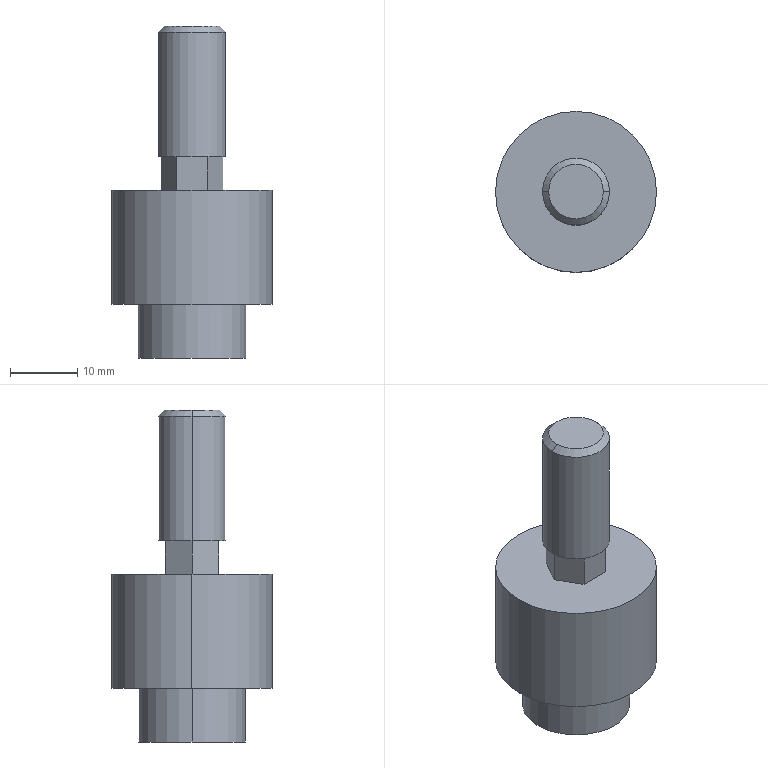Part | STEP file | Bag feed JA30-10-125 floating joint | 1 solid | 24 faces | box 24 x 24 x 49.5 mm | volume 10590 mm3 | plane 12 | cylinder 8 | cone 4 | commonest cylinder face diameters 8.38 x2 10 x2 16 x2 24 x2